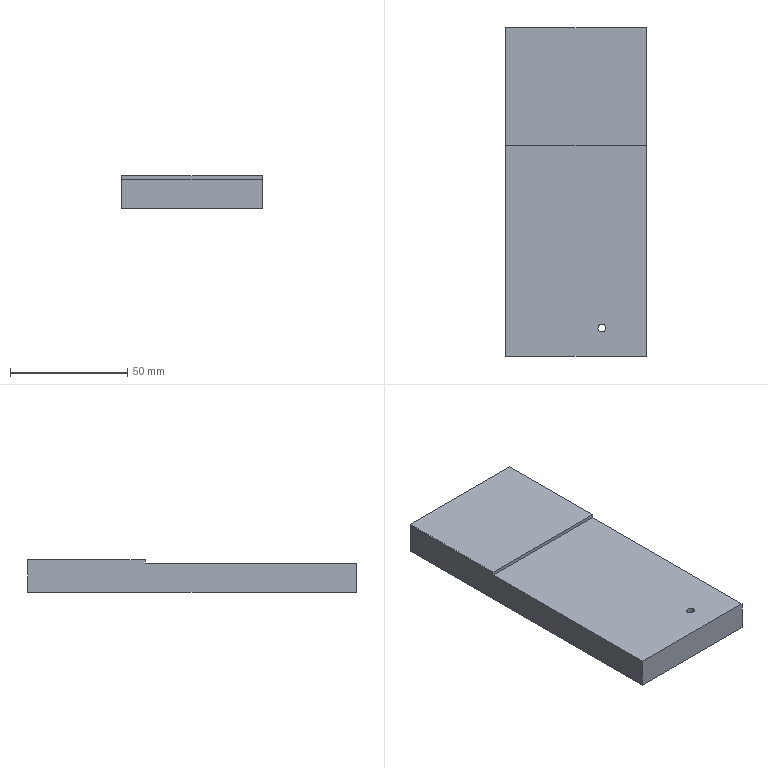Part | SolidWorks | features ICE 2, Cut 1, Extrusion 1, Fillet 1, HoleWzd 1 | 1 solid | 10 faces | box 60 x 140 x 14 mm | volume 109393 mm3 | plane 8 | cylinder 2 | commonest cylinder face diameters 3.3 x2
STEP:
#1=CARTESIAN_POINT('',(12.65,-58.,12.5));
#2=VERTEX_POINT('',#1);
#3=CARTESIAN_POINT('',(9.35,-58.,12.5));
#4=VERTEX_POINT('',#3);
#5=CARTESIAN_POINT('',(11.,-58.,12.5));
#6=DIRECTION('',(0.,0.,-1.));
#7=DIRECTION('',(-1.,0.,0.));
#8=AXIS2_PLACEMENT_3D('',#5,#6,#7);
#9=CIRCLE('',#8,1.65);
#10=EDGE_CURVE('',#2,#4,#9,.T.);
#11=ORIENTED_EDGE('',*,*,#10,.F.);
#12=CARTESIAN_POINT('',(12.65,-58.,0.));
#13=VERTEX_POINT('',#12);
#14=CARTESIAN_POINT('',(12.65,-58.,0.));
#15=DIRECTION('',(0.,0.,-1.));
#16=VECTOR('',#15,1000.);
#17=LINE('',#14,#16);
#18=EDGE_CURVE('',#2,#13,#17,.T.);
#19=ORIENTED_EDGE('',*,*,#18,.T.);
#20=CARTESIAN_POINT('',(9.35,-58.,0.));
#21=VERTEX_POINT('',#20);
#22=CARTESIAN_POINT('',(11.,-58.,0.));
#23=DIRECTION('',(0.,0.,-1.));
#24=DIRECTION('',(-1.,0.,0.));
#25=AXIS2_PLACEMENT_3D('',#22,#23,#24);
#26=CIRCLE('',#25,1.65);
#27=EDGE_CURVE('',#13,#21,#26,.T.);
#28=ORIENTED_EDGE('',*,*,#27,.T.);
#29=CARTESIAN_POINT('',(9.35,-58.,0.));
#30=DIRECTION('',(0.,0.,-1.));
#31=VECTOR('',#30,1000.);
#32=LINE('',#29,#31);
#33=EDGE_CURVE('',#4,#21,#32,.T.);
#34=ORIENTED_EDGE('',*,*,#33,.F.);
#35=EDGE_LOOP('',(#11,#19,#28,#34));
#36=FACE_OUTER_BOUND('',#35,.T.);
#37=CARTESIAN_POINT('',(11.,-58.,0.));
#38=DIRECTION('',(0.,0.,-1.));
#39=DIRECTION('',(-1.,0.,0.));
#40=AXIS2_PLACEMENT_3D('',#37,#38,#39);
#41=CYLINDRICAL_SURFACE('',#40,1.65);
#42=ADVANCED_FACE('',(#36),#41,.F.);
#43=CARTESIAN_POINT('',(30.,20.,14.));
#44=VERTEX_POINT('',#43);
#45=CARTESIAN_POINT('',(30.,70.,14.));
#46=VERTEX_POINT('',#45);
#47=CARTESIAN_POINT('',(30.,-70.,14.));
#48=DIRECTION('',(0.,1.,0.));
#49=VECTOR('',#48,1000.);
#50=LINE('',#47,#49);
#51=EDGE_CURVE('',#44,#46,#50,.T.);
#52=ORIENTED_EDGE('',*,*,#51,.F.);
#53=CARTESIAN_POINT('',(30.,20.,12.5));
#54=VERTEX_POINT('',#53);
#55=CARTESIAN_POINT('',(30.,20.,12.5));
#56=DIRECTION('',(0.,0.,1.));
#57=VECTOR('',#56,1000.);
#58=LINE('',#55,#57);
#59=EDGE_CURVE('',#54,#44,#58,.T.);
#60=ORIENTED_EDGE('',*,*,#59,.F.);
#61=CARTESIAN_POINT('',(30.,-70.,12.5));
#62=VERTEX_POINT('',#61);
#63=CARTESIAN_POINT('',(30.,-70.,12.5));
#64=DIRECTION('',(0.,1.,0.));
#65=VECTOR('',#64,1000.);
#66=LINE('',#63,#65);
#67=EDGE_CURVE('',#62,#54,#66,.T.);
#68=ORIENTED_EDGE('',*,*,#67,.F.);
#69=CARTESIAN_POINT('',(30.,-70.,0.));
#70=VERTEX_POINT('',#69);
#71=CARTESIAN_POINT('',(30.,-70.,14.));
#72=DIRECTION('',(0.,0.,-1.));
#73=VECTOR('',#72,1000.);
#74=LINE('',#71,#73);
#75=EDGE_CURVE('',#62,#70,#74,.T.);
#76=ORIENTED_EDGE('',*,*,#75,.T.);
#77=CARTESIAN_POINT('',(30.,70.,0.));
#78=VERTEX_POINT('',#77);
#79=CARTESIAN_POINT('',(30.,-70.,0.));
#80=DIRECTION('',(0.,1.,0.));
#81=VECTOR('',#80,1000.);
#82=LINE('',#79,#81);
#83=EDGE_CURVE('',#70,#78,#82,.T.);
#84=ORIENTED_EDGE('',*,*,#83,.T.);
#85=CARTESIAN_POINT('',(30.,70.,14.));
#86=DIRECTION('',(0.,0.,-1.));
#87=VECTOR('',#86,1000.);
#88=LINE('',#85,#87);
#89=EDGE_CURVE('',#46,#78,#88,.T.);
#90=ORIENTED_EDGE('',*,*,#89,.F.);
#91=EDGE_LOOP('',(#52,#60,#68,#76,#84,#90));
#92=FACE_OUTER_BOUND('',#91,.T.);
#93=CARTESIAN_POINT('',(30.,-70.,14.));
#94=DIRECTION('',(-1.,0.,0.));
#95=DIRECTION('',(0.,0.,1.));
#96=AXIS2_PLACEMENT_3D('',#93,#94,#95);
#97=PLANE('',#96);
#98=ADVANCED_FACE('',(#92),#97,.F.);
#99=CARTESIAN_POINT('',(-30.,70.,0.));
#100=VERTEX_POINT('',#99);
#101=CARTESIAN_POINT('',(-30.,70.,0.));
#102=DIRECTION('',(-1.,0.,0.));
#103=VECTOR('',#102,1000.);
#104=LINE('',#101,#103);
#105=EDGE_CURVE('',#78,#100,#104,.T.);
#106=ORIENTED_EDGE('',*,*,#105,.T.);
#107=CARTESIAN_POINT('',(-30.,70.,14.));
#108=VERTEX_POINT('',#107);
#109=CARTESIAN_POINT('',(-30.,70.,14.));
#110=DIRECTION('',(0.,0.,-1.));
#111=VECTOR('',#110,1000.);
#112=LINE('',#109,#111);
#113=EDGE_CURVE('',#108,#100,#112,.T.);
#114=ORIENTED_EDGE('',*,*,#113,.F.);
#115=CARTESIAN_POINT('',(-30.,70.,14.));
#116=DIRECTION('',(-1.,0.,0.));
#117=VECTOR('',#116,1000.);
#118=LINE('',#115,#117);
#119=EDGE_CURVE('',#46,#108,#118,.T.);
#120=ORIENTED_EDGE('',*,*,#119,.F.);
#121=ORIENTED_EDGE('',*,*,#89,.T.);
#122=EDGE_LOOP('',(#106,#114,#120,#121));
#123=FACE_OUTER_BOUND('',#122,.T.);
#124=CARTESIAN_POINT('',(-30.,70.,14.));
#125=DIRECTION('',(0.,-1.,0.));
#126=DIRECTION('',(0.,0.,-1.));
#127=AXIS2_PLACEMENT_3D('',#124,#125,#126);
#128=PLANE('',#127);
#129=ADVANCED_FACE('',(#123),#128,.F.);
#130=CARTESIAN_POINT('',(-30.,20.,12.5));
#131=VERTEX_POINT('',#130);
#132=CARTESIAN_POINT('',(-30.,-70.,12.5));
#133=VERTEX_POINT('',#132);
#134=CARTESIAN_POINT('',(-30.,-70.,12.5));
#135=DIRECTION('',(0.,-1.,0.));
#136=VECTOR('',#135,1000.);
#137=LINE('',#134,#136);
#138=EDGE_CURVE('',#131,#133,#137,.T.);
#139=ORIENTED_EDGE('',*,*,#138,.F.);
#140=CARTESIAN_POINT('',(-30.,20.,14.));
#141=VERTEX_POINT('',#140);
#142=CARTESIAN_POINT('',(-30.,20.,12.5));
#143=DIRECTION('',(0.,0.,1.));
#144=VECTOR('',#143,1000.);
#145=LINE('',#142,#144);
#146=EDGE_CURVE('',#131,#141,#145,.T.);
#147=ORIENTED_EDGE('',*,*,#146,.T.);
#148=CARTESIAN_POINT('',(-30.,-70.,14.));
#149=DIRECTION('',(0.,-1.,0.));
#150=VECTOR('',#149,1000.);
#151=LINE('',#148,#150);
#152=EDGE_CURVE('',#108,#141,#151,.T.);
#153=ORIENTED_EDGE('',*,*,#152,.F.);
#154=ORIENTED_EDGE('',*,*,#113,.T.);
#155=CARTESIAN_POINT('',(-30.,-70.,0.));
#156=VERTEX_POINT('',#155);
#157=CARTESIAN_POINT('',(-30.,-70.,0.));
#158=DIRECTION('',(0.,-1.,0.));
#159=VECTOR('',#158,1000.);
#160=LINE('',#157,#159);
#161=EDGE_CURVE('',#100,#156,#160,.T.);
#162=ORIENTED_EDGE('',*,*,#161,.T.);
#163=CARTESIAN_POINT('',(-30.,-70.,14.));
#164=DIRECTION('',(0.,0.,-1.));
#165=VECTOR('',#164,1000.);
#166=LINE('',#163,#165);
#167=EDGE_CURVE('',#133,#156,#166,.T.);
#168=ORIENTED_EDGE('',*,*,#167,.F.);
#169=EDGE_LOOP('',(#139,#147,#153,#154,#162,#168));
#170=FACE_OUTER_BOUND('',#169,.T.);
#171=CARTESIAN_POINT('',(-30.,-70.,14.));
#172=DIRECTION('',(1.,0.,0.));
#173=DIRECTION('',(0.,0.,-1.));
#174=AXIS2_PLACEMENT_3D('',#171,#172,#173);
#175=PLANE('',#174);
#176=ADVANCED_FACE('',(#170),#175,.F.);
#177=ORIENTED_EDGE('',*,*,#75,.F.);
#178=CARTESIAN_POINT('',(-30.,-70.,12.5));
#179=DIRECTION('',(1.,0.,0.));
#180=VECTOR('',#179,1000.);
#181=LINE('',#178,#180);
#182=EDGE_CURVE('',#133,#62,#181,.T.);
#183=ORIENTED_EDGE('',*,*,#182,.F.);
#184=ORIENTED_EDGE('',*,*,#167,.T.);
#185=CARTESIAN_POINT('',(-30.,-70.,0.));
#186=DIRECTION('',(1.,0.,0.));
#187=VECTOR('',#186,1000.);
#188=LINE('',#185,#187);
#189=EDGE_CURVE('',#156,#70,#188,.T.);
#190=ORIENTED_EDGE('',*,*,#189,.T.);
#191=EDGE_LOOP('',(#177,#183,#184,#190));
#192=FACE_OUTER_BOUND('',#191,.T.);
#193=CARTESIAN_POINT('',(-30.,-70.,14.));
#194=DIRECTION('',(0.,1.,0.));
#195=DIRECTION('',(0.,0.,1.));
#196=AXIS2_PLACEMENT_3D('',#193,#194,#195);
#197=PLANE('',#196);
#198=ADVANCED_FACE('',(#192),#197,.F.);
#199=ORIENTED_EDGE('',*,*,#152,.T.);
#200=CARTESIAN_POINT('',(-30.,20.,14.));
#201=DIRECTION('',(-1.,0.,0.));
#202=VECTOR('',#201,1000.);
#203=LINE('',#200,#202);
#204=EDGE_CURVE('',#44,#141,#203,.T.);
#205=ORIENTED_EDGE('',*,*,#204,.F.);
#206=ORIENTED_EDGE('',*,*,#51,.T.);
#207=ORIENTED_EDGE('',*,*,#119,.T.);
#208=EDGE_LOOP('',(#199,#205,#206,#207));
#209=FACE_OUTER_BOUND('',#208,.T.);
#210=CARTESIAN_POINT('',(0.,0.,14.));
#211=DIRECTION('',(0.,0.,-1.));
#212=DIRECTION('',(-1.,0.,0.));
#213=AXIS2_PLACEMENT_3D('',#210,#211,#212);
#214=PLANE('',#213);
#215=ADVANCED_FACE('',(#209),#214,.F.);
#216=CARTESIAN_POINT('',(11.,-58.,0.));
#217=DIRECTION('',(0.,0.,-1.));
#218=DIRECTION('',(-1.,0.,0.));
#219=AXIS2_PLACEMENT_3D('',#216,#217,#218);
#220=CIRCLE('',#219,1.65);
#221=EDGE_CURVE('',#21,#13,#220,.T.);
#222=ORIENTED_EDGE('',*,*,#221,.F.);
#223=ORIENTED_EDGE('',*,*,#27,.F.);
#224=EDGE_LOOP('',(#222,#223));
#225=FACE_BOUND('',#224,.T.);
#226=ORIENTED_EDGE('',*,*,#83,.F.);
#227=ORIENTED_EDGE('',*,*,#189,.F.);
#228=ORIENTED_EDGE('',*,*,#161,.F.);
#229=ORIENTED_EDGE('',*,*,#105,.F.);
#230=EDGE_LOOP('',(#226,#227,#228,#229));
#231=FACE_OUTER_BOUND('',#230,.T.);
#232=CARTESIAN_POINT('',(0.,0.,0.));
#233=DIRECTION('',(0.,0.,-1.));
#234=DIRECTION('',(-1.,0.,0.));
#235=AXIS2_PLACEMENT_3D('',#232,#233,#234);
#236=PLANE('',#235);
#237=ADVANCED_FACE('',(#225,#231),#236,.T.);
#238=ORIENTED_EDGE('',*,*,#204,.T.);
#239=ORIENTED_EDGE('',*,*,#146,.F.);
#240=CARTESIAN_POINT('',(-30.,20.,12.5));
#241=DIRECTION('',(-1.,0.,0.));
#242=VECTOR('',#241,1000.);
#243=LINE('',#240,#242);
#244=EDGE_CURVE('',#54,#131,#243,.T.);
#245=ORIENTED_EDGE('',*,*,#244,.F.);
#246=ORIENTED_EDGE('',*,*,#59,.T.);
#247=EDGE_LOOP('',(#238,#239,#245,#246));
#248=FACE_OUTER_BOUND('',#247,.T.);
#249=CARTESIAN_POINT('',(-30.,20.,12.5));
#250=DIRECTION('',(0.,1.,0.));
#251=DIRECTION('',(0.,0.,1.));
#252=AXIS2_PLACEMENT_3D('',#249,#250,#251);
#253=PLANE('',#252);
#254=ADVANCED_FACE('',(#248),#253,.F.);
#255=CARTESIAN_POINT('',(11.,-58.,12.5));
#256=DIRECTION('',(0.,0.,-1.));
#257=DIRECTION('',(-1.,0.,0.));
#258=AXIS2_PLACEMENT_3D('',#255,#256,#257);
#259=CIRCLE('',#258,1.65);
#260=EDGE_CURVE('',#4,#2,#259,.T.);
#261=ORIENTED_EDGE('',*,*,#260,.T.);
#262=ORIENTED_EDGE('',*,*,#10,.T.);
#263=EDGE_LOOP('',(#261,#262));
#264=FACE_BOUND('',#263,.T.);
#265=ORIENTED_EDGE('',*,*,#138,.T.);
#266=ORIENTED_EDGE('',*,*,#182,.T.);
#267=ORIENTED_EDGE('',*,*,#67,.T.);
#268=ORIENTED_EDGE('',*,*,#244,.T.);
#269=EDGE_LOOP('',(#265,#266,#267,#268));
#270=FACE_OUTER_BOUND('',#269,.T.);
#271=CARTESIAN_POINT('',(0.,0.,12.5));
#272=DIRECTION('',(0.,0.,-1.));
#273=DIRECTION('',(-1.,0.,0.));
#274=AXIS2_PLACEMENT_3D('',#271,#272,#273);
#275=PLANE('',#274);
#276=ADVANCED_FACE('',(#264,#270),#275,.F.);
#277=ORIENTED_EDGE('',*,*,#18,.F.);
#278=ORIENTED_EDGE('',*,*,#260,.F.);
#279=ORIENTED_EDGE('',*,*,#33,.T.);
#280=ORIENTED_EDGE('',*,*,#221,.T.);
#281=EDGE_LOOP('',(#277,#278,#279,#280));
#282=FACE_OUTER_BOUND('',#281,.T.);
#283=CARTESIAN_POINT('',(11.,-58.,0.));
#284=DIRECTION('',(0.,0.,-1.));
#285=DIRECTION('',(-1.,0.,0.));
#286=AXIS2_PLACEMENT_3D('',#283,#284,#285);
#287=CYLINDRICAL_SURFACE('',#286,1.65);
#288=ADVANCED_FACE('',(#282),#287,.F.);
#289=CLOSED_SHELL('',(#42,#98,#129,#176,#198,#215,#237,#254,#276,#288));
#290=MANIFOLD_SOLID_BREP('',#289);
#291=CARTESIAN_POINT('',(0.,0.,0.));
#292=DIRECTION('',(0.,0.,1.));
#293=DIRECTION('',(1.,0.,0.));
#294=AXIS2_PLACEMENT_3D('',#291,#292,#293);
#295=(LENGTH_UNIT()NAMED_UNIT(*)SI_UNIT(.MILLI.,.METRE.));
#296=UNCERTAINTY_MEASURE_WITH_UNIT(LENGTH_MEASURE(0.00001),#295,'','');
#297=(NAMED_UNIT(*)PLANE_ANGLE_UNIT()SI_UNIT($,.RADIAN.));
#298=(NAMED_UNIT(*)SI_UNIT($,.STERADIAN.)SOLID_ANGLE_UNIT());
#299=(GEOMETRIC_REPRESENTATION_CONTEXT(3)GLOBAL_UNCERTAINTY_ASSIGNED_CONTEXT((#296))GLOBAL_UNIT_ASSIGNED_CONTEXT((#295,#297,#298))REPRESENTATION_CONTEXT('',''));
#300=ADVANCED_BREP_SHAPE_REPRESENTATION('',(#290,#294),#299);